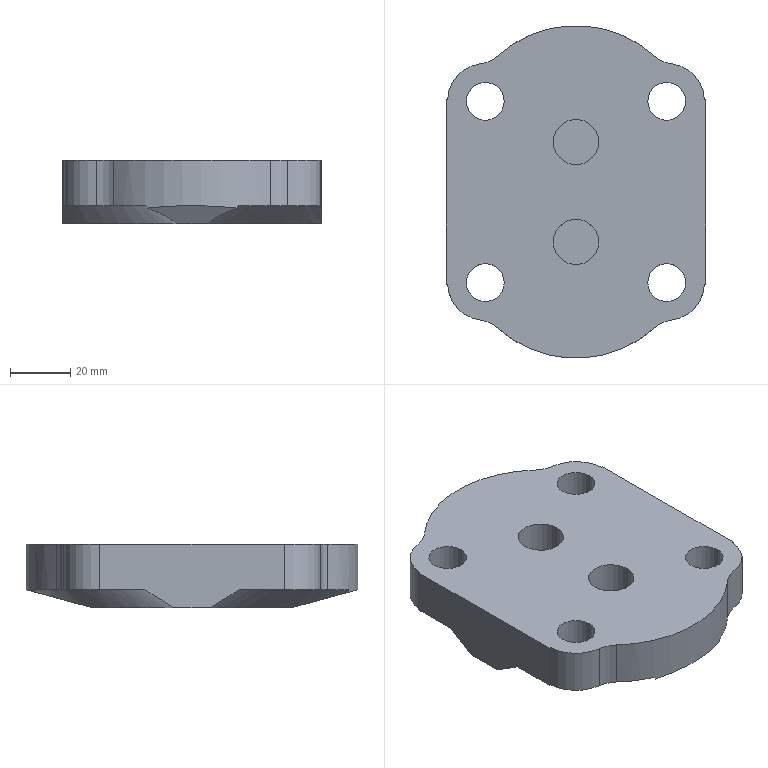Part | SolidWorks | features ICE 7, Split 3, HoleWzd 2, MirrorPattern 2, BlendCut 1, Extrusion 1, Fillet 1, MirrorSolid 1, MoveFace 1 | 1 solid | 52 faces | box 86 x 110 x 21 mm | volume 130372 mm3 | cylinder 27 | plane 21 | spline 4 | commonest cylinder face diameters 12.5 x8 8 x5 15 x4 20 x4 25 x4 77 x2